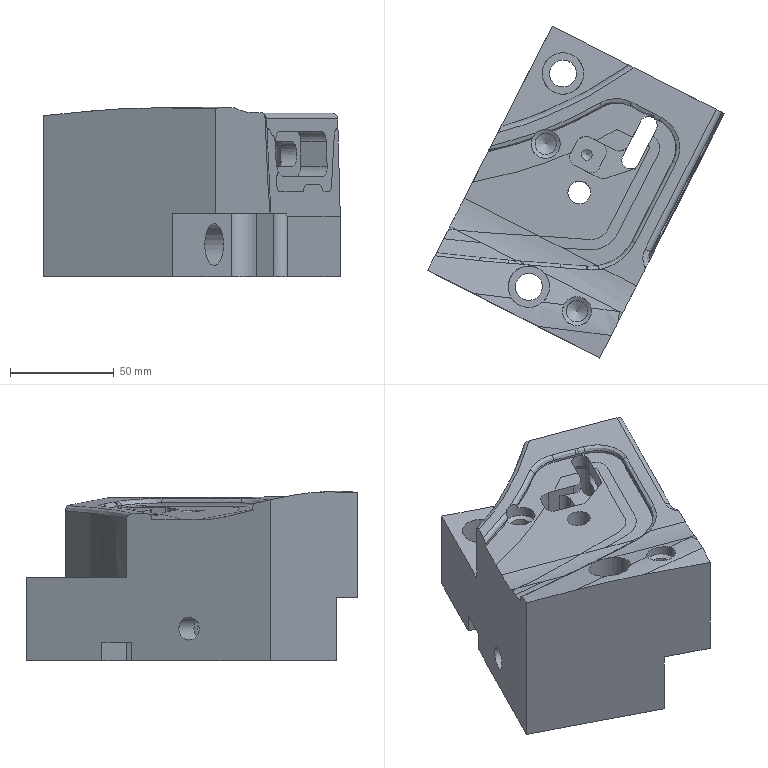Part | STEP file | gslz 2016.10.28-13_id258_x_t | 1 solid | 139 faces | box 142.791 x 159.834 x 81.664 mm | volume 688741 mm3 | plane 45 | spline 36 | cylinder 36 | other 16 | cone 6 | commonest cylinder face diameters 8.4 x7 10 x4 16 x3 20 x3 8 x2 10.3 x2